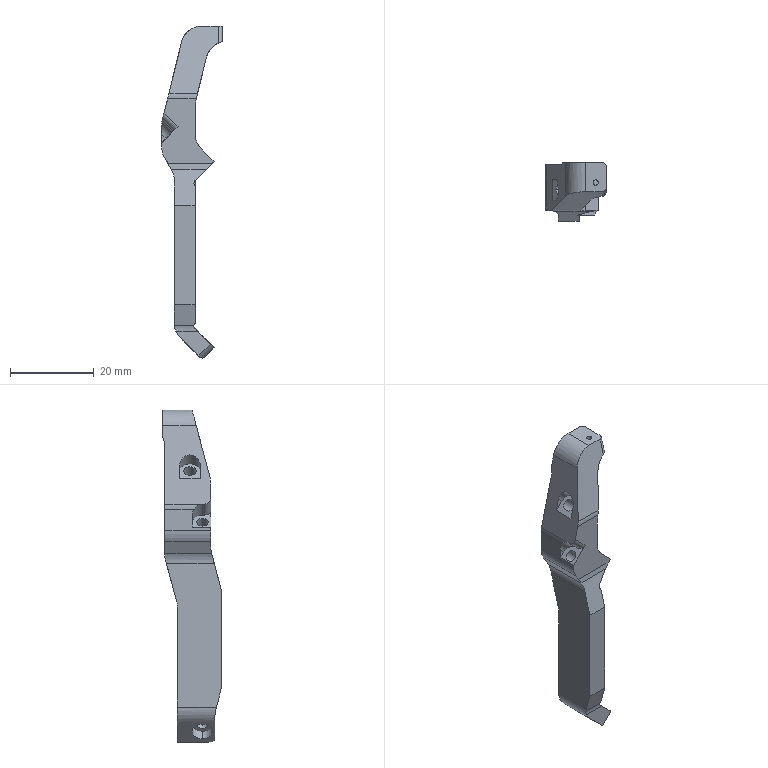NC program | NX | posted by the shop | part box 14.5 x 14 x 79.438 mm
Lines 9635 to 10667 of 13169:
T02 M6 ( D6-18-D6-50-3T-rough )
M41
M51
G90 G54 G00 B90. C90.
M40
M50
G54 G00 X-169.254 Y16.502 S4500 M03
G43 H02 Z-134.89 M08
Z-171.29
G01 X-169.278 Y16.495 Z-171.446 F1500.
X-169.303 Y16.489 Z-171.508
X-169.327 Y16.482 Z-171.553
X-169.351 Y16.476 Z-171.59
X-169.375 Y16.469 Z-171.621
X-169.399 Y16.463 Z-171.647
X-169.423 Y16.456 Z-171.67
X-169.447 Y16.45 Z-171.69
X-169.472 Y16.443 Z-171.708
X-169.496 Y16.437 Z-171.723
X-169.52 Y16.43 Z-171.737
X-169.544 Y16.424 Z-171.748
X-169.568 Y16.417 Z-171.758
X-169.592 Y16.411 Z-171.767
X-169.616 Y16.404 Z-171.774
X-169.641 Y16.398 Z-171.78
X-169.665 Y16.391 Z-171.784
X-169.689 Y16.385 Z-171.787
X-169.713 Y16.378 Z-171.789
X-169.737 Y16.372 Z-171.79
X-171.165 Y15.988
G03 X-171.614 Y15.402 R0.606
X-171.1 Y14.803 R0.606
X-168.749 Y14.611 R14.457
X-168.369 Y14.616 R14.457
X-166.784 Y14.698 R16.779
G02 X-164.162 Y14.577 R38.642
X-161.823 Y13.378 R5.126
G03 X-161.394 Y13.092 R1.956
G01 X-161.244 Y13.072
G03 X-160.644 Y13.672 R0.6
X-160.889 Y14.156 R0.6
X-161.256 Y14.283 Z-171.757 R0.773
G01 X-162.045 Y14.418 Z-171.69
X-162.621 Y14.516 F9999.
X-163.797 Y14.716 Z-171.79 F1500.
X-170.997 Y15.942
X-171.097 Y15.95
G03 X-171.697 Y15.35 R0.6
X-171.335 Y14.8 R0.6
X-170.339 Y14.578 R13.401
G01 X-166.024 Y14.577
G02 X-162.343 Y13.388 R7.513
G03 X-161.275 Y12.903 R4.154
G01 X-161.26 Y12.902
X-161.233 Y12.901
G03 X-160.622 Y13.512 R0.611
X-160.936 Y14.047 R0.611
G01 X-162.042 Y14.494 Z-171.69
X-162.97 Y14.866 F9999.
X-164.078 Y15.309 Z-171.79 F1500.
X-164.914 Y15.644
G03 X-165.141 Y15.688 R0.611
X-165.753 Y15.076 R0.611
X-165.345 Y14.5 R0.611
G02 X-162.236 Y13.109 R23.023
G03 X-161.163 Y12.803 R2.548
X-160.63 Y13.413 R0.615
X-160.954 Y13.954 R0.615
G01 X-162.045 Y14.438 Z-171.69
X-162.935 Y14.83 F9999.
X-164.026 Y15.312 Z-171.79 F1500.
G03 X-164.362 Y15.403 R0.664
X-164.708 Y15.305 R0.664
X-164.985 Y14.791 R0.615
X-164.7 Y14.272 R0.615
X-161.817 Y12.799 R12.073
X-161.241 Y12.721 R2.157
G01 X-161.111 Y12.725
G03 X-160.636 Y13.312 R0.6
X-160.959 Y13.844 R0.6
G01 X-162.054 Y14.318 Z-171.69
X-162.709 Y14.601 F9999.
X-163.668 Y15.009 Z-171.777 F1500.
X-163.817 Y15.032 Z-171.79
X-163.834
G03 X-164.434 Y14.432 R0.6
X-164.156 Y13.926 R0.6
X-161.491 Y12.635 R5.094
G01 X-161.387 Y12.634
G03 X-161.087 Y12.646 R3.86
X-160.642 Y13.225 R0.6
X-160.967 Y13.758 R0.6
G01 X-162.06 Y14.237 Z-171.69
X-162.571 Y14.46 F9999.
X-163.029 Y14.663 Z-171.732 F1500.
X-163.493 Y14.854 Z-171.774
X-163.587 Y14.867 Z-171.782
X-163.681 Y14.871 Z-171.79
G03 X-164.243 Y14.273 R0.6
X-164.07 Y13.852 R0.6
X-161.227 Y12.538 R3.788
G01 X-161.065 Y12.568
G03 X-160.645 Y13.162 R0.63
X-160.963 Y13.709 R0.63
G01 X-162.064 Y14.165 Z-171.69
X-162.453 Y14.324 F9999.
X-162.821 Y14.477 Z-171.723 F1500.
X-163.193 Y14.618 Z-171.757
X-163.335 Y14.634 Z-171.769
G03 X-163.582 Y14.586 Z-171.79 R0.657
X-163.967 Y14.005 R0.63
X-163.786 Y13.563 R0.63
X-161.444 Y12.459 R3.036
X-161.079 Y12.481 R3.036
G01 X-161.051 Y12.491
G03 X-160.653 Y13.056 R0.6
X-160.957 Y13.578 R0.6
G01 X-161.378 Y13.743 Z-171.752
X-161.806 Y13.892 Z-171.714
X-162.076 Y13.99 Z-171.69
X-162.283 Y14.064 F9999.
X-162.652 Y14.2 Z-171.723 F1500.
X-163.027 Y14.323 Z-171.756
X-163.128 Y14.331 Z-171.765
G03 X-163.419 Y14.259 Z-171.79 R0.624
X-163.732 Y13.732 R0.6
X-163.643 Y13.418 R0.6
X-161.84 Y12.381 R2.567
X-161.531 Y12.36 R2.297
X-161.046 Y12.412 R2.297
X-160.657 Y12.986 R0.619
X-160.965 Y13.521 R0.619
G01 X-161.385 Y13.692 Z-171.752
X-161.811 Y13.846 Z-171.714
X-162.079 Y13.946 Z-171.69
X-162.25 Y14.01 F9999.
X-162.59 Y14.139 Z-171.721 F1500.
X-162.934 Y14.258 Z-171.751
X-163.058 Y14.27 Z-171.762
G03 X-163.382 Y14.182 Z-171.79 R0.636
X-163.68 Y13.652 R0.619
X-163.588 Y13.328 R0.619
X-161.835 Y12.288 R2.33
X-161.565 Y12.27 R2.068
X-161.025 Y12.342 R2.068
X-160.663 Y12.893 R0.6
X-160.966 Y13.414 R0.6
G01 X-161.335 Y13.558 Z-171.757
X-161.71 Y13.686 Z-171.724
X-162.088 Y13.82 Z-171.69
X-162.145 Y13.84 F9999.
X-162.515 Y13.974 Z-171.723 F1500.
X-162.889 Y14.093 Z-171.756
X-162.986 Y14.101 Z-171.764
G03 X-163.282 Y14.026 Z-171.79 R0.623
X-163.59 Y13.502 R0.6
X-163.502 Y13.188 R0.6
X-161.758 Y12.191 R2.173
G01 X-161.595 Y12.184
G03 X-161.016 Y12.269 R2.019
X-160.668 Y12.814 R0.6
X-161.081 Y13.384 R0.6
G01 X-162.709 Y13.919
X-162.806 Y13.971
X-162.896 Y13.949
G03 X-163.496 Y13.349 R0.6
X-163.407 Y13.034 R0.6
X-161.737 Y12.104 R2.031
G01 X-161.618 Y12.1
G03 X-161.007 Y12.199 R1.948
X-160.673 Y12.737 R0.6
X-161.101 Y13.311 R0.6
G01 X-162.63 Y13.77
X-162.802 Y13.795
G03 X-163.402 Y13.195 R0.6
X-163.313 Y12.881 R0.6
X-161.712 Y12.019 R1.917
G01 X-161.67
X-161.634
G03 X-160.998 Y12.13 R1.866
X-160.678 Y12.661 R0.6
X-161.129 Y13.242 R0.6
G01 X-162.568 Y13.61
X-162.717 Y13.629
G03 X-163.317 Y13.029 R0.6
G01 X-163.285 Y12.835
G03 X-162.117 Y11.995 R1.599
X-161.659 Y11.939 R1.895
X-161.001 Y12.057 R1.895
X-160.681 Y12.601 R0.623
X-161.128 Y13.198 R0.623
G01 X-162.51 Y13.605
X-162.686 Y13.63
G03 X-163.309 Y13.008 R0.623
X-163.275 Y12.807 R0.623
X-162.211 Y11.941 R1.471
X-161.674 Y11.861 R1.847
X-160.99 Y11.992 R1.847
X-160.687 Y12.522 R0.615
X-161.13 Y13.113 R0.615
G01 X-162.492 Y13.511
X-162.664 Y13.535
G03 X-163.279 Y12.92 R0.615
X-163.246 Y12.721 R0.615
X-162.189 Y11.858 R1.442
X-161.683 Y11.785 R1.775
X-160.979 Y11.93 R1.775
X-160.692 Y12.442 R0.6
X-161.132 Y13.02 R0.6
G01 X-162.484 Y13.394
X-162.644 Y13.416
G03 X-163.244 Y12.816 R0.6
G01 X-163.212 Y12.622
G03 X-162.09 Y11.759 R1.449
X-161.684 Y11.71 R1.719
X-160.985 Y11.859 R1.719
X-160.696 Y12.385 R0.623
X-161.152 Y12.985 R0.623
G01 X-162.428 Y13.338
X-162.594 Y13.361
G03 X-163.216 Y12.738 R0.623
X-163.183 Y12.537 R0.623
X-162.099 Y11.688 R1.402
X-161.692 Y11.637 R1.655
X-160.97 Y11.802 R1.655
X-160.701 Y12.302 R0.6
X-161.152 Y12.883 R0.6
G01 X-162.432 Y13.213
X-162.581 Y13.231
G03 X-163.181 Y12.631 R0.6
G01 X-163.149 Y12.437
G03 X-162.032 Y11.601 R1.399
X-161.693 Y11.565 R1.598
X-160.964 Y11.741 R1.598
X-160.706 Y12.234 R0.6
X-161.16 Y12.816 R0.6
G01 X-162.406 Y13.128
X-162.552 Y13.146
G03 X-163.152 Y12.546 R0.6
G01 X-163.12 Y12.352
G03 X-161.99 Y11.523 R1.376
X-161.695 Y11.495 R1.57
X-160.969 Y11.673 R1.57
X-160.708 Y12.179 R0.623
X-161.182 Y12.783 R0.623
G01 X-162.352 Y13.073
X-162.502 Y13.091
G03 X-163.124 Y12.468 R0.623
X-163.091 Y12.267 R0.623
X-161.937 Y11.445 R1.358
X-161.693 Y11.425 R1.51
X-160.961 Y11.615 R1.51
X-160.714 Y12.1 R0.6
X-161.178 Y12.684 R0.6
G01 X-162.357 Y12.96
X-162.494 Y12.976
G03 X-163.094 Y12.376 R0.6
G01 X-163.062 Y12.182
G03 X-161.924 Y11.375 R1.327
X-161.695 Y11.357 R1.482
X-160.961 Y11.552 R1.482
X-160.718 Y12.044 R0.619
X-161.199 Y12.647 R0.619
G01 X-162.31 Y12.9
X-162.447 Y12.916
G03 X-163.066 Y12.297 R0.619
X-163.033 Y12.097 R0.619
X-161.9 Y11.305 R1.302
X-161.694 Y11.29 R1.431
X-160.951 Y11.498 R1.431
X-160.721 Y11.972 R0.604
X-161.226 Y12.567 R0.604
G01 X-162.322 Y12.75
X-162.421 Y12.758
G03 X-163.025 Y12.154 R0.604
G01 X-163.015 Y12.045
G03 X-162.038 Y11.263 R1.201
X-161.705 Y11.223 R1.443
X-160.955 Y11.433 R1.443
X-160.725 Y11.916 R0.623
X-161.232 Y12.528 R0.623
G01 X-162.281 Y12.726
X-162.396 Y12.737
G03 X-163.019 Y12.115 R0.623
G01 X-163.015 Y12.045
G03 X-162.225 Y11.25 R1.075
X-161.717 Y11.157 R1.443
X-160.947 Y11.38 R1.443
X-160.73 Y11.844 R0.604
X-161.203 Y12.433 R0.604
G01 X-162.281 Y12.672
X-162.412 Y12.687
G03 X-163.016 Y12.083 R0.604
G01 X-163.012 Y12.015
G03 X-162.237 Y11.19 R1.056
X-161.719 Y11.093 R1.421
X-160.945 Y11.323 R1.421
X-160.734 Y11.781 R0.604
X-161.204 Y12.37 R0.604
G01 X-162.272 Y12.612
X-162.405 Y12.627
G03 X-163.009 Y12.023 R0.604
G01 X-163.005 Y11.956
G03 X-162.222 Y11.123 R1.06
X-161.719 Y11.03 R1.407
X-160.953 Y11.257 R1.407
X-160.737 Y11.733 R0.634
X-161.235 Y12.352 R0.634
G01 X-162.231 Y12.571
X-162.367 Y12.586
G03 X-163.001 Y11.952 R0.634
G01 X-162.997 Y11.881
G03 X-162.169 Y11.042 R1.082
X-161.718 Y10.966 R1.374
X-160.949 Y11.202 R1.374
X-160.741 Y11.669 R0.63
X-161.233 Y12.284 R0.63
G01 X-162.226 Y12.507
X-162.364 Y12.522
G03 X-162.994 Y11.892 R0.63
G01 X-162.99 Y11.822
G03 X-162.156 Y10.976 R1.081
X-161.719 Y10.904 R1.35
X-160.946 Y11.146 R1.35
X-160.746 Y11.606 R0.626
X-161.232 Y12.216 R0.626
G01 X-162.221 Y12.442
X-162.361 Y12.458
G03 X-162.987 Y11.832 R0.626
G01 X-162.983 Y11.762
G03 X-162.16 Y10.916 R1.073
X-161.721 Y10.841 R1.329
X-160.94 Y11.095 R1.329
X-160.75 Y11.535 R0.604
X-161.227 Y12.125 R0.604
G01 X-162.248 Y12.345
X-162.375 Y12.359
G03 X-162.979 Y11.755 R0.604
G01 X-162.975 Y11.688
G03 X-162.104 Y10.838 R1.087
X-161.719 Y10.78 R1.298
X-160.936 Y11.042 R1.298
X-160.754 Y11.475 R0.604
X-161.229 Y12.065 R0.604
G01 X-162.24 Y12.285
X-162.368 Y12.299
G03 X-162.972 Y11.695 R0.604
G01 X-162.968 Y11.628
G03 X-162.103 Y10.777 R1.079
X-161.721 Y10.719 R1.295
X-160.945 Y10.977 R1.295
X-160.757 Y11.43 R0.638
X-161.255 Y12.052 R0.638
G01 X-161.77 Y12.171
X-162.288 Y12.276
X-162.328 Y12.277
G03 X-162.966 Y11.639 R0.638
G01 X-162.962 Y11.568
G03 X-162.1 Y10.715 R1.071
X-161.723 Y10.658 R1.274
X-160.939 Y10.928 R1.274
X-160.762 Y11.364 R0.626
X-161.258 Y11.977 R0.626
G01 X-161.777 Y12.091
X-162.299 Y12.189
X-162.331 Y12.19
G03 X-162.957 Y11.563 R0.626
G01 X-162.953 Y11.494
G03 X-162.077 Y10.649 R1.074
X-161.722 Y10.598 R1.257
X-160.941 Y10.87 R1.257
X-160.765 Y11.309 R0.634
X-161.266 Y11.929 R0.634
G01 X-161.773 Y12.041
X-162.283 Y12.138
X-162.317 Y12.139
G03 X-162.95 Y11.505 R0.634
G01 X-162.947 Y11.434
G03 X-162.076 Y10.589 R1.065
X-161.724 Y10.538 R1.237
X-160.934 Y10.823 R1.237
X-160.769 Y11.237 R0.604
X-161.248 Y11.828 R0.604
G01 X-162.215 Y12.032
X-162.34 Y12.046
G03 X-162.944 Y11.442 R0.604
G01 X-162.94 Y11.374
G03 X-162.07 Y10.528 R1.058
X-161.724 Y10.478 R1.222
X-160.933 Y10.769 R1.222
X-160.773 Y11.178 R0.604
X-161.26 Y11.77 R0.604
G01 X-162.214 Y11.96
X-162.331 Y11.971
G03 X-162.935 Y11.367 R0.604
G01 X-162.932 Y11.3
G03 X-162.04 Y10.462 R1.064
X-161.723 Y10.419 R1.205
X-160.934 Y10.713 R1.205
X-160.777 Y11.12 R0.604
X-161.263 Y11.712 R0.604
G01 X-162.207 Y11.9
X-162.325 Y11.911
G03 X-162.929 Y11.308 R0.604
G01 X-162.925 Y11.24
G03 X-162.059 Y10.408 R1.047
X-161.726 Y10.361 R1.202
X-160.937 Y10.656 R1.202
X-160.78 Y11.074 R0.634
X-161.313 Y11.7 R0.634
G01 X-161.798 Y11.782
X-162.286 Y11.849
X-162.288
G03 X-162.922 Y11.215 R0.634
X-162.21 Y10.396 R0.97
X-161.74 Y10.301 R1.22
X-160.937 Y10.603 R1.22
X-160.784 Y11.014 R0.63
X-161.294 Y11.633 R0.63
G01 X-161.781 Y11.732
X-162.272 Y11.815
X-162.292
G03 X-162.922 Y11.185 R0.63
X-162.229 Y10.345 R0.956
X-161.743 Y10.242 R1.206
X-160.93 Y10.557 R1.206
X-160.788 Y10.946 R0.604
X-161.268 Y11.537 R0.604
G01 X-161.778 Y11.648
X-162.291 Y11.743
X-162.318 Y11.744
G03 X-162.922 Y11.14 R0.604
X-162.215 Y10.281 R0.958
X-161.744 Y10.185 R1.201
X-160.937 Y10.496 R1.201
X-160.791 Y10.903 R0.641
X-161.301 Y11.531 R0.641
G01 X-161.775 Y11.634
X-162.252 Y11.721
X-162.281
G03 X-162.922 Y11.08 R0.641
X-162.237 Y10.232 R0.956
X-161.747 Y10.127 R1.194
X-160.936 Y10.445 R1.194
X-160.795 Y10.845 R0.638
X-161.304 Y11.469 R0.638
G01 X-161.779 Y11.571
X-162.258 Y11.657
X-162.284 Y11.658
G03 X-162.922 Y11.02 R0.638
X-162.226 Y10.17 R0.961
X-161.748 Y10.069 R1.18
X-160.933 Y10.396 R1.18
X-160.799 Y10.784 R0.63
X-161.303 Y11.402 R0.63
G01 X-161.784 Y11.503
X-162.267 Y11.59
X-162.292
G03 X-162.922 Y10.96 R0.63
X-162.219 Y10.11 R0.963
X-161.749 Y10.011 R1.165
X-160.929 Y10.349 R1.165
X-160.803 Y10.718 R0.604
X-161.279 Y11.308 R0.604
G01 X-161.782 Y11.421
X-162.287 Y11.518
X-162.318 Y11.519
G03 X-162.922 Y10.915 R0.604
X-162.206 Y10.047 R0.963
X-161.75 Y9.954 R1.158
X-160.932 Y10.293 R1.158
X-160.806 Y10.68 R0.656
X-161.322 Y11.321 R0.656
G01 X-161.775 Y11.424
X-162.232 Y11.511
X-162.266
G03 X-162.922 Y10.855 R0.656
X-162.18 Y9.981 R0.974
X-161.75 Y9.898 R1.15
X-160.935 Y10.236 R1.15
X-160.81 Y10.616 R0.638
X-161.314 Y11.239 R0.638
G01 X-161.782 Y11.343
X-162.253 Y11.432
X-162.284 Y11.433
G03 X-162.922 Y10.795 R0.638
X-162.22 Y9.938 R0.961
X-161.756 Y9.84 R1.148
X-160.932 Y10.188 R1.148
X-160.813 Y10.558 R0.634
X-161.316 Y11.178 R0.634
G01 X-161.786 Y11.281
X-162.259 Y11.368
X-162.288 Y11.369
G03 X-162.922 Y10.735 R0.634
X-162.216 Y9.879 R0.962
X-161.758 Y9.783 R1.144
X-160.935 Y10.133 R1.144
X-160.817 Y10.503 R0.641
X-161.327 Y11.131 R0.641
G01 X-161.788 Y11.231
X-162.252 Y11.316
X-162.281
G03 X-162.922 Y10.675 R0.641
X-162.253 Y9.837 R0.945
X-161.762 Y9.726 R1.145
X-160.936 Y10.079 R1.145
X-160.821 Y10.445 R0.641
X-161.332 Y11.073 R0.641
G01 X-161.791 Y11.172
X-162.253 Y11.256
X-162.281
G03 X-162.922 Y10.615 R0.641
X-162.21 Y9.763 R0.961
X-161.76 Y9.669 R1.119
X-160.929 Y10.038 R1.119
X-160.825 Y10.376 R0.604
X-161.301 Y10.966 R0.604
G01 X-161.792 Y11.077
X-162.287 Y11.173
X-162.318 Y11.174
G03 X-162.922 Y10.57 R0.604
X-162.21 Y9.707 R0.955
X-161.761 Y9.613 R1.121
X-160.936 Y9.976 R1.121
X-160.829 Y10.33 R0.638
X-161.329 Y10.952 R0.638
G01 X-161.788 Y11.057
X-162.25 Y11.147
X-162.284 Y11.148
G03 X-162.922 Y10.51 R0.638
X-162.171 Y9.637 R0.969
X-161.759 Y9.557 R1.104
X-160.935 Y9.927 R1.104
X-160.832 Y10.274 R0.638
X-161.335 Y10.897 R0.638
G01 X-161.792 Y11.
X-162.252 Y11.087
X-162.284 Y11.088
G03 X-162.922 Y10.45 R0.638
X-162.221 Y9.598 R0.954
X-161.766 Y9.5 R1.108
X-160.936 Y9.873 R1.108
X-160.836 Y10.216 R0.638
X-161.34 Y10.84 R0.638
G01 X-161.795 Y10.941
X-162.253 Y11.027
X-162.284 Y11.028
G03 X-162.922 Y10.39 R0.638
X-162.217 Y9.54 R0.953
X-161.767 Y9.444 R1.106
X-160.941 Y9.815 R1.106
G01 X-160.933 Y9.827
G03 X-160.84 Y10.149 R0.604
X-161.321 Y10.74 R0.604
G01 X-161.805 Y10.844
X-162.292 Y10.933
X-162.318 Y10.934
G03 X-162.922 Y10.33 R0.604
X-162.214 Y9.482 R0.955
X-161.769 Y9.388 R1.098
X-160.941 Y9.765 R1.098
G01 X-160.933 Y9.778
G03 X-160.844 Y10.093 R0.604
X-161.318 Y10.683 R0.604
G01 X-161.8 Y10.793
X-162.286 Y10.888
X-162.318 Y10.889
G03 X-162.922 Y10.285 R0.604
X-162.215 Y9.426 R0.948
X-161.77 Y9.331 R1.089
X-160.939 Y9.717 R1.089
X-160.847 Y10.051 R0.649
X-161.353 Y10.684 R0.649
G01 X-161.793 Y10.786
X-162.236 Y10.873
X-162.273 Y10.874
G03 X-162.922 Y10.225 R0.649
X-162.22 Y9.372 R0.948
X-161.773 Y9.276 R1.09
X-160.944 Y9.658 R1.09
G01 X-160.937 Y9.67
G03 X-160.85 Y9.998 R0.66
X-161.366 Y10.642 R0.66
G01 X-161.794 Y10.741
X-162.225 Y10.824
X-162.262 Y10.825
G03 X-162.922 Y10.165 R0.66
X-162.172 Y9.299 R0.963
X-161.769 Y9.221 R1.074
X-160.947 Y9.603 R1.074
G01 X-160.939 Y9.616
G03 X-160.854 Y9.937 R0.645
X-161.363 Y10.567 R0.645
G01 X-161.802 Y10.666
X-162.244 Y10.749
X-162.277 Y10.75
G03 X-162.922 Y10.105 R0.645
X-162.164 Y9.24 R0.966
X-161.769 Y9.165 R1.062
X-160.944 Y9.558 R1.062
G01 X-160.937 Y9.571
G03 X-160.858 Y9.869 R0.604
X-161.34 Y10.46 R0.604
G01 X-161.815 Y10.562
X-162.293 Y10.648
X-162.318 Y10.649
G03 X-162.922 Y10.045 R0.604
X-162.218 Y9.203 R0.947
X-161.779 Y9.11 R1.086
X-160.958 Y9.485 R1.086
G01 X-160.943 Y9.511
G03 X-160.861 Y9.828 R0.656
X-161.37 Y10.468 R0.656
G01 X-161.796 Y10.569
X-162.225 Y10.655
X-162.266 Y10.656
G03 X-162.922 Y10. R0.656
X-162.254 Y9.16 R0.927
X-161.786 Y9.055 R1.097
X-160.966 Y9.423 R1.097
G01 X-160.943 Y9.462
G03 X-160.865 Y9.771 R0.649
X-161.372 Y10.404 R0.649
G01 X-161.803 Y10.504
X-162.237 Y10.588
X-162.273 Y10.589
G03 X-162.922 Y9.94 R0.649
X-162.176 Y9.077 R0.954
X-161.778 Y8.999 R1.06
X-160.957 Y9.388 R1.06
G01 X-160.942 Y9.414
G03 X-160.868 Y9.716 R0.653
X-161.381 Y10.353 R0.653
G01 X-161.806 Y10.45
X-162.234 Y10.532
X-162.269 Y10.533
G03 X-162.922 Y9.88 R0.653
X-162.168 Y9.018 R0.958
X-161.778 Y8.943 R1.05
X-160.957 Y9.339 R1.05
G01 X-160.942 Y9.365
G03 X-160.872 Y9.648 R0.608
X-161.357 Y10.243 R0.608
G01 X-161.822 Y10.342
X-162.289 Y10.427
X-162.314 Y10.428
G03 X-162.922 Y9.82 R0.608
X-162.209 Y8.976 R0.942
X-161.787 Y8.889 R1.067
X-160.967 Y9.273 R1.067
G01 X-160.945 Y9.312
G03 X-160.875 Y9.605 R0.653
X-161.382 Y10.241 R0.653
G01 X-161.804 Y10.342
X-162.229 Y10.426
X-162.269 Y10.428
G03 X-162.922 Y9.775 R0.653
X-162.258 Y8.938 R0.92
X-161.794 Y8.835 R1.085
X-160.978 Y9.205 R1.085
G01 X-160.948 Y9.256
G03 X-160.879 Y9.549 R0.653
X-161.388 Y10.185 R0.653
G01 X-161.808 Y10.283
X-162.231 Y10.367
X-162.269 Y10.368
G03 X-162.922 Y9.715 R0.653
X-162.22 Y8.869 R0.936
X-161.791 Y8.779 R1.068
X-160.978 Y9.156 R1.068
G01 X-160.948 Y9.208
G03 X-160.883 Y9.492 R0.649
X-161.392 Y10.125 R0.649
G01 X-161.813 Y10.222
X-162.238 Y10.303
X-162.273 Y10.304
G03 X-162.922 Y9.655 R0.649
X-162.172 Y8.798 R0.951
X-161.787 Y8.724 R1.045
X-160.973 Y9.115 R1.045
G01 X-160.951 Y9.154
G03 X-160.886 Y9.44 R0.66
X-161.407 Y10.085 R0.66
G01 X-161.816 Y10.177
X-162.228 Y10.254
X-162.262 Y10.255
G03 X-162.922 Y9.595 R0.66
X-162.164 Y8.74 R0.953
X-161.787 Y8.669 R1.037
X-160.974 Y9.063 R1.037
G01 X-160.946 Y9.117
G03 X-160.89 Y9.371 R0.608
X-161.368 Y9.964 R0.608
G01 X-161.823 Y10.068
X-162.282 Y10.157
X-162.314 Y10.158
G03 X-162.922 Y9.55 R0.608
X-162.209 Y8.7 R0.932
X-161.796 Y8.616 R1.056
X-160.986 Y8.994 R1.056
G01 X-160.951 Y9.06
X-160.929 Y9.228
G03 X-161.349 Y9.843 R0.66
G01 X-161.735 Y9.996
X-162.125 Y10.136
X-162.262 Y10.15
G03 X-162.922 Y9.49 R0.66
X-162.206 Y8.643 R0.931
X-161.798 Y8.562 R1.056
X-160.991 Y8.937 R1.056
G01 X-160.949 Y9.016
G03 X-160.898 Y9.262 R0.608
X-161.381 Y9.856 R0.608
G01 X-161.833 Y9.954
X-162.288 Y10.037
X-162.314 Y10.038
G03 X-162.922 Y9.43 R0.608
X-162.166 Y8.576 R0.946
X-161.794 Y8.506 R1.03
X-160.985 Y8.899 R1.03
G01 X-160.951 Y8.966
G03 X-160.901 Y9.207 R0.608
X-161.388 Y9.802 R0.608
G01 X-161.838 Y9.897
X-162.291 Y9.977
X-162.314 Y9.978
G03 X-162.922 Y9.37 R0.608
X-162.173 Y8.523 R0.946
X-161.797 Y8.452 R1.033
X-160.991 Y8.839 R1.033
G01 X-160.957 Y8.905
G03 X-160.904 Y9.163 R0.66
X-161.415 Y9.806 R0.66
G01 X-161.816 Y9.902
X-162.22 Y9.984
X-162.262 Y9.985
G03 X-162.922 Y9.325 R0.66
X-162.222 Y8.484 R0.925
X-161.806 Y8.398 R1.043
X-160.995 Y8.784 R1.043
G01 X-160.955 Y8.864
G03 X-160.908 Y9.098 R0.608
X-161.391 Y9.692 R0.608
G01 X-161.838 Y9.789
X-162.287 Y9.872
X-162.314 Y9.873
G03 X-162.922 Y9.265 R0.608
X-162.214 Y8.427 R0.927
X-161.807 Y8.343 R1.037
X-160.996 Y8.734 R1.037
G01 X-160.956 Y8.815
G03 X-160.912 Y9.043 R0.608
X-161.398 Y9.639 R0.608
G01 X-161.843 Y9.733
X-162.29 Y9.812
X-162.314 Y9.813
G03 X-162.922 Y9.205 R0.608
X-162.171 Y8.359 R0.941
X-161.803 Y8.29 R1.023
X-161. Y8.679 R1.023
G01 X-160.96 Y8.76
G03 X-160.915 Y8.989 R0.608
X-161.394 Y9.582 R0.608
G01 X-161.837 Y9.682
X-162.283 Y9.767
X-162.314 Y9.768
G03 X-162.922 Y9.16 R0.608
X-162.216 Y8.318 R0.925
X-161.811 Y8.235 R1.034
X-161.005 Y8.622 R1.034
G01 X-160.965 Y8.702
G03 X-160.919 Y8.943 R0.66
X-161.431 Y9.587 R0.66
G01 X-161.825 Y9.68
X-162.221 Y9.759
X-162.262 Y9.76
G03 X-162.922 Y9.1 R0.66
X-162.208 Y8.261 R0.926
X-161.812 Y8.182 R1.033
X-161.011 Y8.562 R1.033
G01 X-160.965 Y8.656
G03 X-160.927 Y8.875 R0.66
X-161.431 Y9.517 R0.66
G01 X-161.82 Y9.615
X-162.213 Y9.698
X-162.262 Y9.7
G03 X-162.922 Y9.04 R0.66
X-162.218 Y8.21 R0.921
X-161.815 Y8.129 R1.037
X-161.018 Y8.502 R1.037
G01 X-160.965 Y8.609
G03 X-160.926 Y8.824 R0.608
X-161.404 Y9.418 R0.608
G01 X-161.841 Y9.517
X-162.282 Y9.602
X-162.314 Y9.603
G03 X-162.922 Y8.995 R0.608
X-162.17 Y8.141 R0.933
X-161.81 Y8.075 R1.017
X-161.017 Y8.456 R1.017
G01 X-160.965 Y8.564
G03 X-160.929 Y8.771 R0.611
X-161.413 Y9.368 R0.611
G01 X-161.846 Y9.464
X-162.281 Y9.546
X-162.311
G03 X-162.922 Y8.935 R0.611
X-162.245 Y8.111 R0.907
X-161.822 Y8.021 R1.041
X-161.028 Y8.389 R1.041
G01 X-160.969 Y8.51
G03 X-160.933 Y8.717 R0.611
X-161.421 Y9.316 R0.611
G01 X-161.852 Y9.408
X-162.285 Y9.486
X-162.311
G03 X-162.922 Y8.875 R0.611
X-162.172 Y8.033 R0.933
X-161.813 Y7.967 R1.005
X-161.018 Y8.358 R1.005
G01 X-160.973 Y8.453
G03 X-160.937 Y8.67 R0.66
X-161.443 Y9.312 R0.66
G01 X-161.827 Y9.408
X-162.215 Y9.489
X-162.262 Y9.49
G03 X-162.922 Y8.83 R0.66
X-162.169 Y7.978 R0.931
X-161.815 Y7.913 R1.001
X-161.021 Y8.305 R1.001
G01 X-160.972 Y8.415
X-160.943 Y8.481
X-160.94 Y8.609
G03 X-161.424 Y9.207 R0.611
G01 X-161.852 Y9.301
X-162.282 Y9.381
X-162.311
G03 X-162.922 Y8.77 R0.611
X-162.213 Y7.938 R0.917
X-161.824 Y7.861 R1.021
X-161.033 Y8.236 R1.021
G01 X-160.976 Y8.358
G03 X-160.944 Y8.563 R0.66
X-161.459 Y9.207 R0.66
G01 X-161.84 Y9.295
X-162.224 Y9.369
X-162.262 Y9.37
G03 X-162.922 Y8.71 R0.66
X-162.166 Y7.87 R0.932
X-161.818 Y7.806 R0.99
X-161.023 Y8.207 R0.99
G01 X-160.976 Y8.317
X-160.947 Y8.502
G03 X-161.428 Y9.099 R0.611
G01 X-161.852 Y9.194
X-162.279 Y9.276
X-162.311
G03 X-162.922 Y8.665 R0.611
X-162.163 Y7.815 R0.931
X-161.82 Y7.754 R0.991
X-161.03 Y8.147 R0.991
G01 X-160.977 Y8.27
X-160.95 Y8.448
G03 X-161.436 Y9.047 R0.611
G01 X-161.858 Y9.138
X-162.283 Y9.216
X-162.311
G03 X-162.922 Y8.605 R0.611
X-162.211 Y7.776 R0.914
X-161.829 Y7.7 R1.002
X-161.035 Y8.091 R1.002
G01 X-160.981 Y8.215
X-160.954 Y8.395
G03 X-161.444 Y8.994 R0.611
G01 X-161.865 Y9.082
X-162.287 Y9.156
X-162.311
G03 X-162.922 Y8.545 R0.611
X-162.165 Y7.709 R0.93
X-161.823 Y7.647 R0.981
X-161.032 Y8.049 R0.981
G01 X-160.985 Y8.16
X-160.958 Y8.347
G03 X-161.465 Y8.99 R0.66
G01 X-161.839 Y9.081
X-162.217 Y9.159
X-162.262 Y9.16
G03 X-162.922 Y8.5 R0.66
X-162.208 Y7.668 R0.914
X-161.832 Y7.594 R0.995
X-161.04 Y7.988 R0.995
G01 X-160.987 Y8.112
X-160.961 Y8.294
G03 X-161.475 Y8.938 R0.66
G01 X-161.847 Y9.025
X-162.222 Y9.099
X-162.262 Y9.1
G03 X-162.922 Y8.44 R0.66
X-162.214 Y7.617 R0.91
X-161.835 Y7.542 R0.995
X-161.044 Y7.933 R0.995
G01 X-160.987 Y8.071
X-160.964 Y8.237
G03 X-161.448 Y8.838 R0.615
G01 X-161.86 Y8.93
X-162.275 Y9.009
X-162.307 Y9.01
G03 X-162.922 Y8.395 R0.615
X-162.172 Y7.551 R0.92
X-161.83 Y7.489 R0.972
X-161.039 Y7.897 R0.972
G01 X-160.989 Y8.022
X-160.968 Y8.183
G03 X-161.456 Y8.785 R0.615
G01 X-161.866 Y8.874
X-162.279 Y8.95
X-162.307
G03 X-162.922 Y8.335 R0.615
X-162.202 Y7.507 R0.912
X-161.837 Y7.436 R0.985
X-161.048 Y7.831 R0.985
G01 X-160.992 Y7.97
X-160.971 Y8.129
G03 X-161.464 Y8.732 R0.615
G01 X-161.872 Y8.818
X-162.283 Y8.89
X-162.307
G03 X-162.922 Y8.275 R0.615
X-162.165 Y7.443 R0.924
X-161.833 Y7.384 R0.972
X-161.05 Y7.78 R0.972
G01 X-160.995 Y7.919
X-160.975 Y8.075
G03 X-161.46 Y8.677 R0.615
G01 X-161.867 Y8.767
X-162.276 Y8.844
X-162.307 Y8.845
G03 X-162.922 Y8.23 R0.615
X-162.162 Y7.389 R0.921
X-161.835 Y7.332 R0.971
X-161.055 Y7.724 R0.971
G01 X-160.999 Y7.863
X-160.979 Y8.024
G03 X-161.488 Y8.667 R0.66
G01 X-161.852 Y8.755
X-162.218 Y8.829
X-162.262 Y8.83
G03 X-162.922 Y8.17 R0.66
X-162.202 Y7.347 R0.909
X-161.843 Y7.279 R0.984
X-161.063 Y7.663 R0.984
G01 X-161.001 Y7.815
X-160.999 Y7.865
G03 X-161.398 Y8.471 R0.661
G01 X-161.748 Y8.625
X-162.104 Y8.766
X-162.262 Y8.785
G03 X-162.922 Y8.125 R0.66
X-162.164 Y7.284 R0.917
X-161.838 Y7.227 R0.963
X-161.059 Y7.625 R0.963
G01 X-161.004 Y7.764
X-160.999 Y7.85
G03 X-161.437 Y8.471 R0.66
G01 X-161.787 Y8.599
X-162.142 Y8.714
X-162.262 Y8.725
G03 X-162.922 Y8.065 R0.66
X-162.157 Y7.229 R0.92
X-161.838 Y7.174 R0.95
X-161.055 Y7.586 R0.95
G01 X-161.007 Y7.712
X-160.989 Y7.867
G03 X-161.489 Y8.507 R0.66
G01 X-161.847 Y8.6
X-162.209 Y8.678
X-162.262 Y8.68
G03 X-162.922 Y8.02 R0.66
X-162.166 Y7.179 R0.914
X-161.841 Y7.122 R0.951
X-161.06 Y7.53 R0.951
G01 X-161.008 Y7.671
X-160.992 Y7.812
G03 X-161.481 Y8.417 R0.619
G01 X-161.876 Y8.504
X-162.273 Y8.578
X-162.303 Y8.579
G03 X-162.922 Y7.96 R0.619
X-162.158 Y7.124 R0.916
X-161.842 Y7.07 R0.947
X-161.063 Y7.479 R0.947
G01 X-161.011 Y7.62
X-160.995 Y7.759
G03 X-161.477 Y8.363 R0.619
G01 X-161.871 Y8.455
X-162.267 Y8.533
X-162.303 Y8.534
G03 X-162.922 Y7.915 R0.619
X-162.192 Y7.081 R0.901
X-161.85 Y7.018 R0.958
X-161.071 Y7.419 R0.958
G01 X-161.013 Y7.573
X-160.999 Y7.707
G03 X-161.487 Y8.312 R0.619
G01 X-161.878 Y8.399
X-162.272 Y8.473
X-162.303 Y8.474
G03 X-162.922 Y7.855 R0.619
X-162.194 Y7.029 R0.901
X-161.852 Y6.966 R0.953
X-161.071 Y7.372 R0.953
G01 X-161.015 Y7.527
X-161.002 Y7.656
G03 X-161.498 Y8.265 R0.623
G01 X-161.885 Y8.348
X-162.273 Y8.417
X-162.299 Y8.418
G03 X-162.922 Y7.795 R0.623
X-162.224 Y6.986 R0.891
X-161.858 Y6.914 R0.963
X-161.078 Y7.312 R0.963
G01 X-161.017 Y7.481
X-161.005 Y7.603
G03 X-161.494 Y8.211 R0.623
G01 X-161.879 Y8.298
X-162.266 Y8.372
X-162.299 Y8.373
G03 X-162.922 Y7.75 R0.623
X-162.182 Y6.922 R0.903
X-161.853 Y6.863 R0.946
X-161.078 Y7.266 R0.946
G01 X-161.019 Y7.436